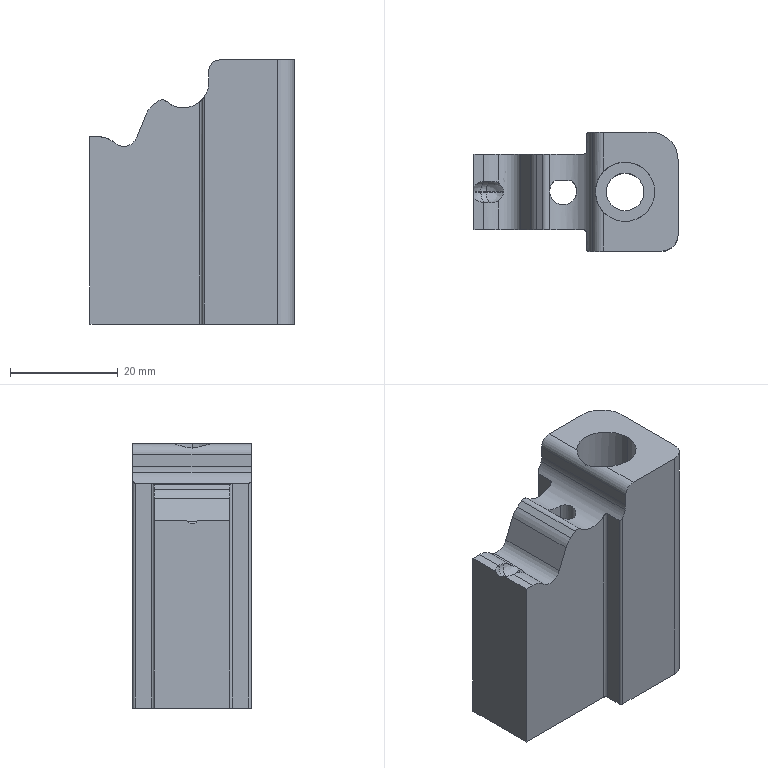Part | 1 solid | 48 faces | box 37.817 x 22 x 48.948 mm | volume 25185 mm3 | cylinder 21 | plane 19 | spline 8 | commonest cylinder face diameters 1 x4 7 x2 8.206 x2 9 x2 9.5 x2 11 x2